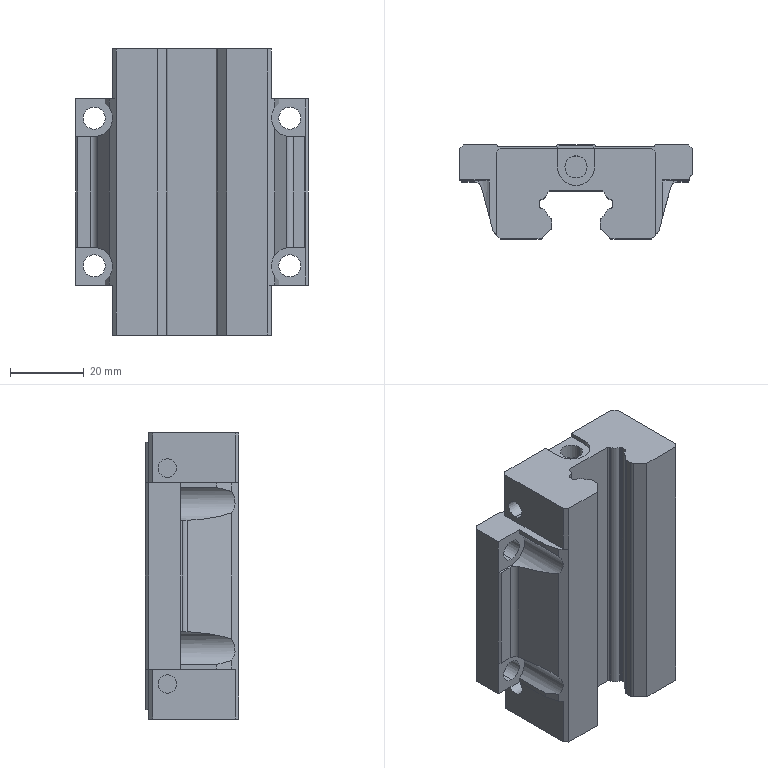Part | SolidWorks | features BaseBody 1 | 1 solid | 166 faces | box 63 x 25.4 x 77.5 mm | volume 76607 mm3 | plane 104 | cylinder 62 | commonest cylinder face diameters 1 x18 6 x12 2 x8 5 x8 10 x6 4.06 x4